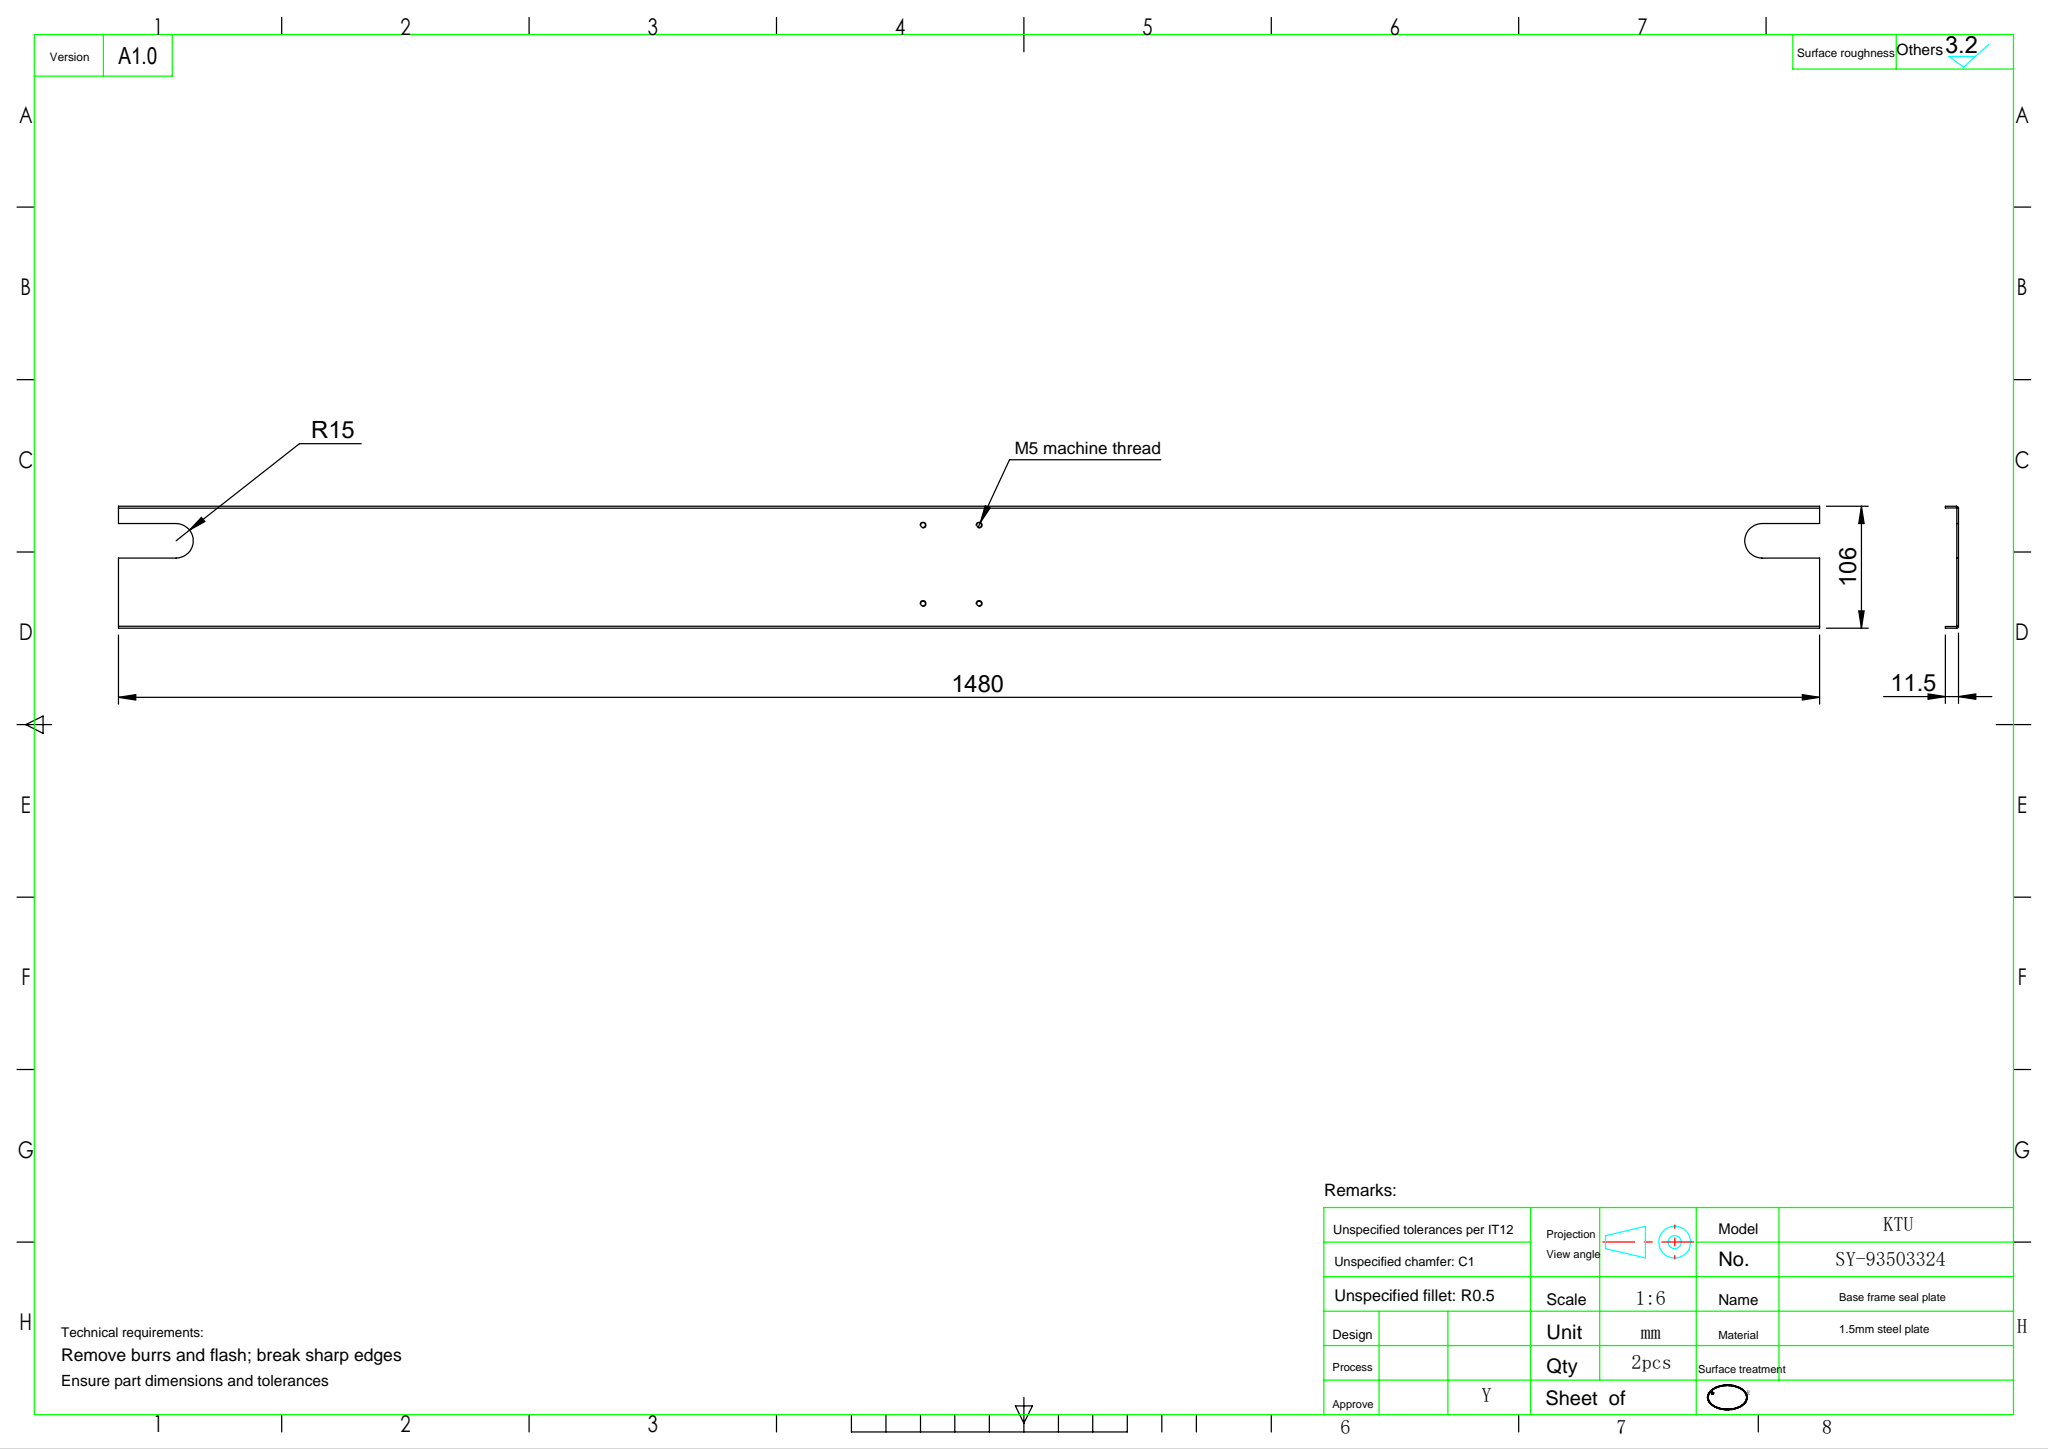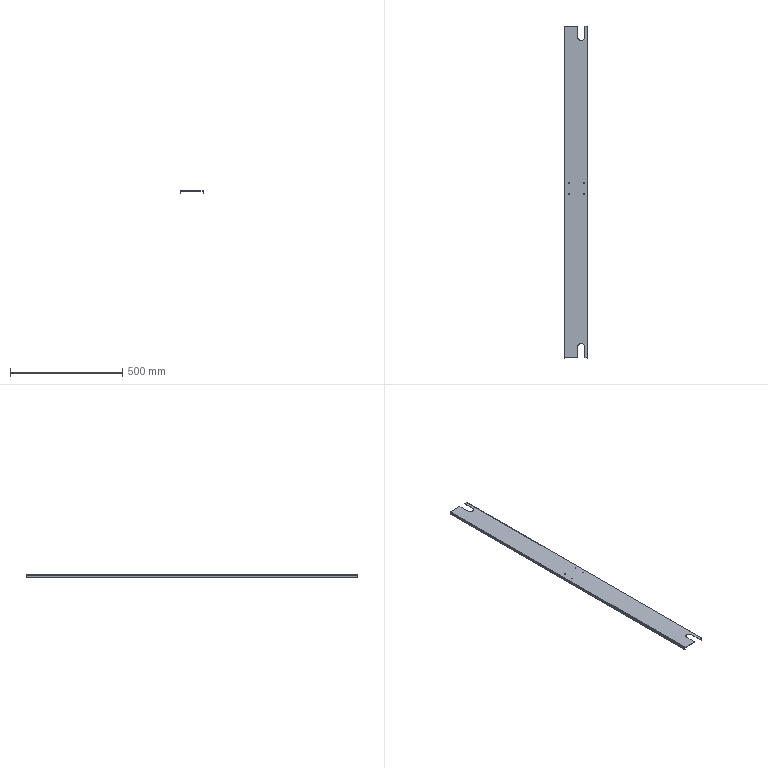Part | SolidWorks | features Cut 2, FlatPattern 1, SMBaseFlange 1, SheetMetal 1 | 1 solid | 38 faces | box 106 x 1480 x 11.5 mm | volume 272266 mm3 | plane 24 | cylinder 14 | commonest cylinder face diameters 4.2 x8 0.4 x2 3.4 x2 30 x2